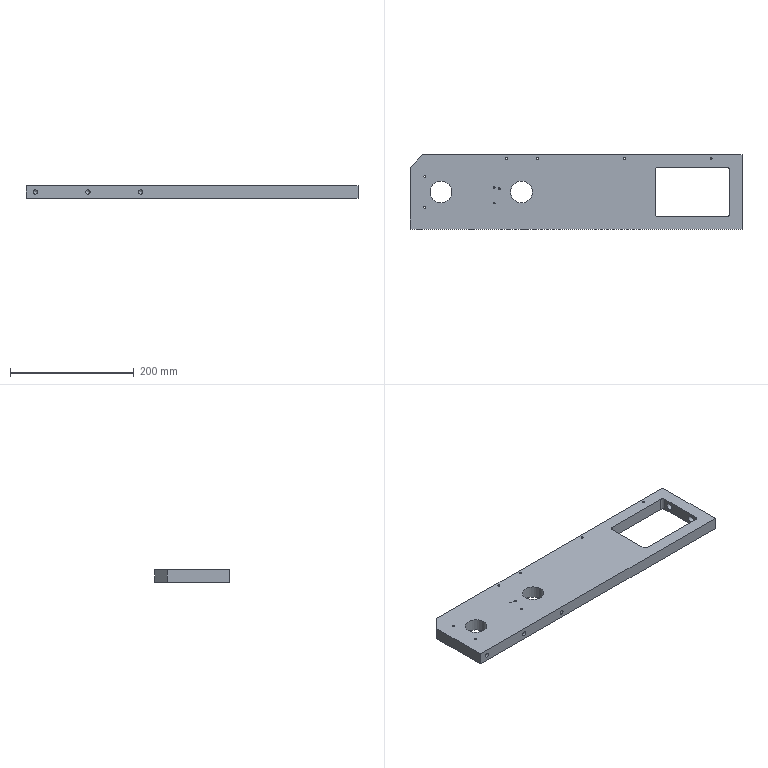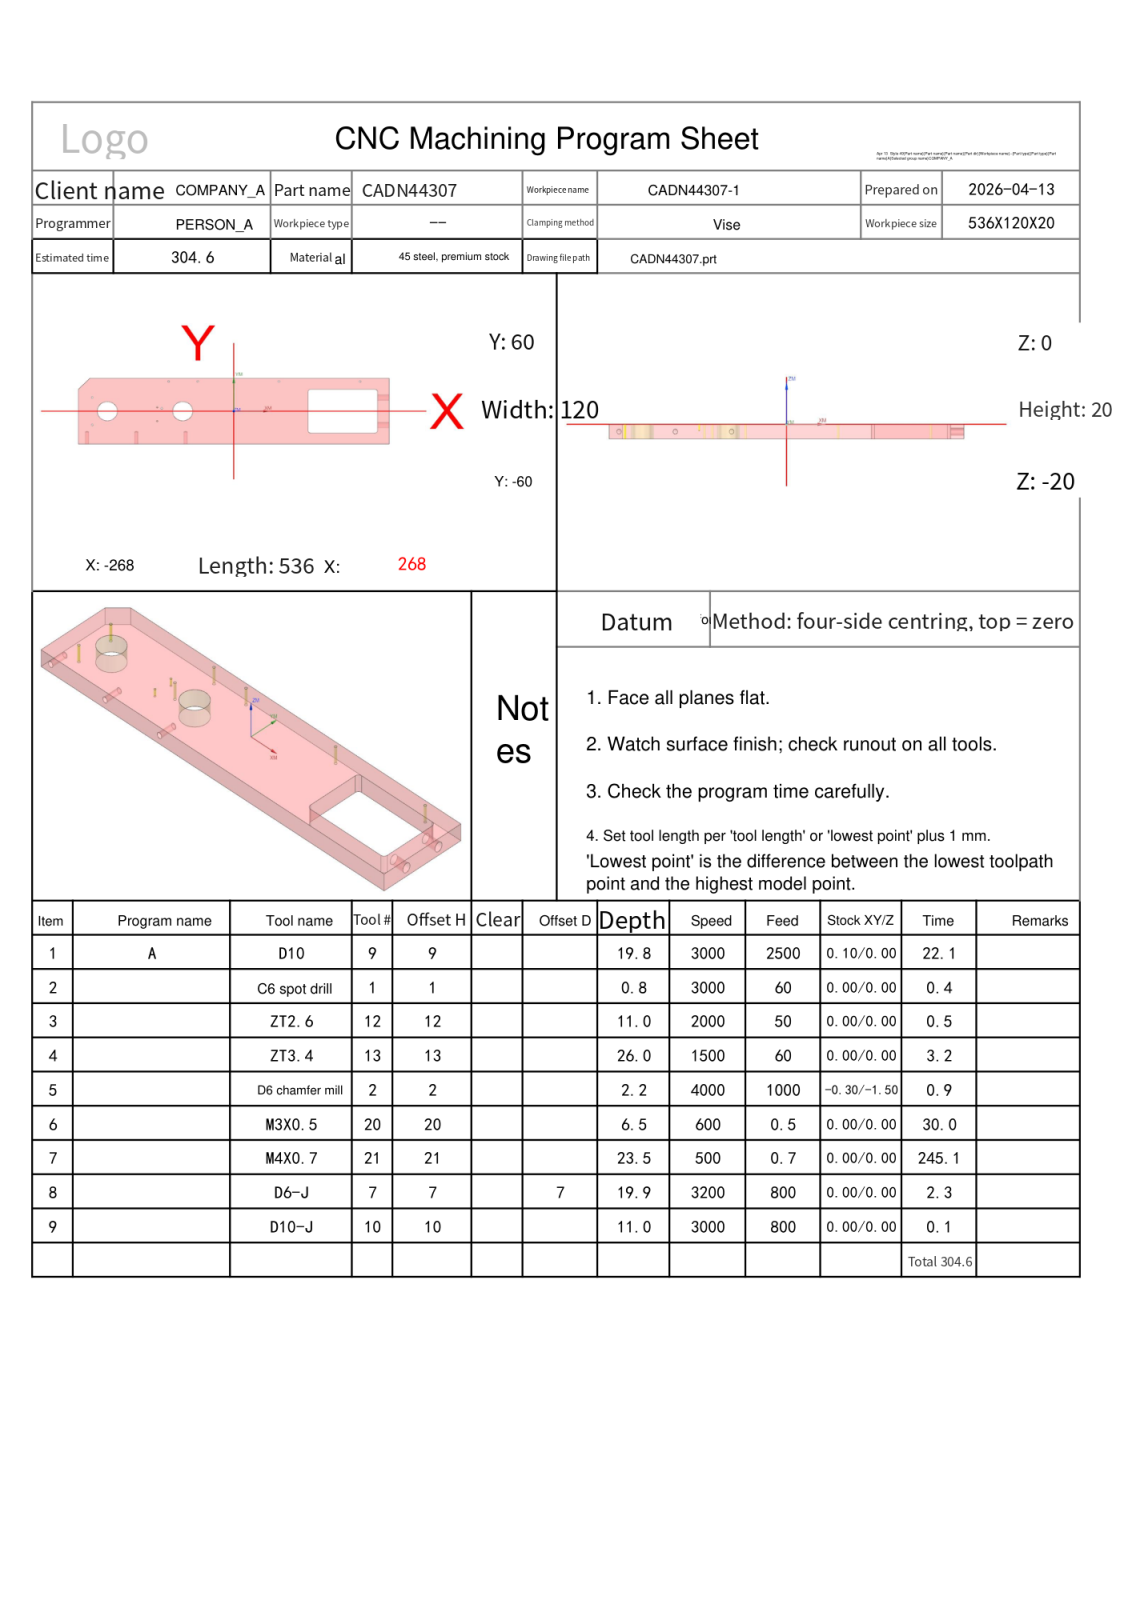NC program | NX | posted by the shop | part box 536 x 120 x 20 mm
Whole program, first 1074 of 1856 lines:
%
O0001
(Machine time: 567.38 MIN)
(===Total Tool:9===)
(T9=D10     D=10.  R=0.   D-  H09 Z=-19.8 )
(T1=C6 spot drill   D=6.   R=0.   D-  H01 Z=-0.8  )
(T12=ZT2.6  D=2.6  DR_a=118 D-  H12 Z=-11.  )
(T13=ZT3.4  D=3.4  DR_a=118 D-  H13 Z=-26.  )
(T2=D6 chamfer mill   D=6.   R=0.   D-  H02 Z=-2.2  )
(T20=M3X0.5 D=2.5  DR_a=180 D-  H20 Z=-6.5  )
(T21=M4X0.7 D=3.3  DR_a=180 D-  H21 Z=-23.5 )
(T7=D6-J    D=6.   R=0.   D7  H07 Z=-19.85)
(T10=D10-J  D=10.  R=0.   D-  H10 Z=-11.  )
G80 G90 G17 G49 G40
G91 G28 Z0
M01
N1 T09 M06
(D10  D=10. R=0. H=09 ce=0.10 di=0.00)
G00 G90 G54 X-230.4 Y0.0 M03 S3000
G43 H09 Z20.
M08
Z.5
G03 X-218. Y-12.4 Z.45 I12.4 J0.0 F2500.
X-205.6 Y0.0 Z.4 I0.0 J12.4
X-218. Y12.4 Z.351 I-12.4 J0.0
X-230.4 Y0.0 Z.301 I0.0 J-12.4
X-218. Y-12.4 Z.251 I12.4 J0.0
X-205.6 Y0.0 Z.201 I0.0 J12.4
X-218. Y12.4 Z.152 I-12.4 J0.0
X-230.4 Y0.0 Z.102 I0.0 J-12.4
X-218. Y-12.4 Z.052 I12.4 J0.0
X-205.6 Y0.0 Z.002 I0.0 J12.4
X-218. Y12.4 Z-.047 I-12.4 J0.0
X-230.4 Y0.0 Z-.097 I0.0 J-12.4
X-218. Y-12.4 Z-.147 I12.4 J0.0
X-205.6 Y0.0 Z-.197 I0.0 J12.4
X-218. Y12.4 Z-.246 I-12.4 J0.0
X-230.4 Y0.0 Z-.296 I0.0 J-12.4
X-218. Y-12.4 Z-.346 I12.4 J0.0
X-205.6 Y0.0 Z-.396 I0.0 J12.4
X-218. Y12.4 Z-.445 I-12.4 J0.0
X-230.4 Y0.0 Z-.495 I0.0 J-12.4
X-218. Y-12.4 Z-.545 I12.4 J0.0
X-205.6 Y0.0 Z-.595 I0.0 J12.4
X-218. Y12.4 Z-.644 I-12.4 J0.0
X-230.4 Y0.0 Z-.694 I0.0 J-12.4
X-218. Y-12.4 Z-.744 I12.4 J0.0
X-205.6 Y0.0 Z-.794 I0.0 J12.4
X-218. Y12.4 Z-.843 I-12.4 J0.0
X-230.4 Y0.0 Z-.893 I0.0 J-12.4
X-218. Y-12.4 Z-.943 I12.4 J0.0
X-205.6 Y0.0 Z-.993 I0.0 J12.4
X-218. Y12.4 Z-1.042 I-12.4 J0.0
X-230.4 Y0.0 Z-1.092 I0.0 J-12.4
X-218. Y-12.4 Z-1.142 I12.4 J0.0
X-205.6 Y0.0 Z-1.192 I0.0 J12.4
X-218. Y12.4 Z-1.241 I-12.4 J0.0
X-230.4 Y0.0 Z-1.291 I0.0 J-12.4
X-218. Y-12.4 Z-1.341 I12.4 J0.0
X-205.6 Y0.0 Z-1.391 I0.0 J12.4
X-218. Y12.4 Z-1.44 I-12.4 J0.0
X-230.4 Y0.0 Z-1.49 I0.0 J-12.4
X-218. Y-12.4 Z-1.54 I12.4 J0.0
X-205.6 Y0.0 Z-1.59 I0.0 J12.4
X-218. Y12.4 Z-1.639 I-12.4 J0.0
X-230.4 Y0.0 Z-1.689 I0.0 J-12.4
X-218. Y-12.4 Z-1.739 I12.4 J0.0
X-205.6 Y0.0 Z-1.789 I0.0 J12.4
X-218. Y12.4 Z-1.838 I-12.4 J0.0
X-230.4 Y0.0 Z-1.888 I0.0 J-12.4
X-218. Y-12.4 Z-1.938 I12.4 J0.0
X-205.6 Y0.0 Z-1.988 I0.0 J12.4
X-218. Y12.4 Z-2.038 I-12.4 J0.0
X-230.4 Y0.0 Z-2.087 I0.0 J-12.4
X-218. Y-12.4 Z-2.137 I12.4 J0.0
X-205.6 Y0.0 Z-2.187 I0.0 J12.4
X-218. Y12.4 Z-2.237 I-12.4 J0.0
X-230.4 Y0.0 Z-2.286 I0.0 J-12.4
X-218. Y-12.4 Z-2.336 I12.4 J0.0
X-205.6 Y0.0 Z-2.386 I0.0 J12.4
X-218. Y12.4 Z-2.436 I-12.4 J0.0
X-230.4 Y0.0 Z-2.485 I0.0 J-12.4
X-218. Y-12.4 Z-2.535 I12.4 J0.0
X-205.6 Y0.0 Z-2.585 I0.0 J12.4
X-218. Y12.4 Z-2.635 I-12.4 J0.0
X-230.4 Y0.0 Z-2.684 I0.0 J-12.4
X-218. Y-12.4 Z-2.734 I12.4 J0.0
X-205.6 Y0.0 Z-2.784 I0.0 J12.4
X-218. Y12.4 Z-2.834 I-12.4 J0.0
X-230.4 Y0.0 Z-2.883 I0.0 J-12.4
X-218. Y-12.4 Z-2.933 I12.4 J0.0
X-205.6 Y0.0 Z-2.983 I0.0 J12.4
X-218. Y12.4 Z-3.033 I-12.4 J0.0
X-230.4 Y0.0 Z-3.082 I0.0 J-12.4
X-218. Y-12.4 Z-3.132 I12.4 J0.0
X-205.6 Y0.0 Z-3.182 I0.0 J12.4
X-218. Y12.4 Z-3.232 I-12.4 J0.0
X-230.4 Y0.0 Z-3.281 I0.0 J-12.4
X-218. Y-12.4 Z-3.331 I12.4 J0.0
X-205.6 Y0.0 Z-3.381 I0.0 J12.4
X-218. Y12.4 Z-3.431 I-12.4 J0.0
X-230.4 Y0.0 Z-3.48 I0.0 J-12.4
X-218. Y-12.4 Z-3.53 I12.4 J0.0
X-205.6 Y0.0 Z-3.58 I0.0 J12.4
X-218. Y12.4 Z-3.63 I-12.4 J0.0
X-230.4 Y0.0 Z-3.679 I0.0 J-12.4
X-218. Y-12.4 Z-3.729 I12.4 J0.0
X-205.6 Y0.0 Z-3.779 I0.0 J12.4
X-218. Y12.4 Z-3.829 I-12.4 J0.0
X-230.4 Y0.0 Z-3.878 I0.0 J-12.4
X-218. Y-12.4 Z-3.928 I12.4 J0.0
X-205.6 Y0.0 Z-3.978 I0.0 J12.4
X-218. Y12.4 Z-4.028 I-12.4 J0.0
X-230.4 Y0.0 Z-4.077 I0.0 J-12.4
X-218. Y-12.4 Z-4.127 I12.4 J0.0
X-205.6 Y0.0 Z-4.177 I0.0 J12.4
X-218. Y12.4 Z-4.227 I-12.4 J0.0
X-230.4 Y0.0 Z-4.276 I0.0 J-12.4
X-218. Y-12.4 Z-4.326 I12.4 J0.0
X-205.6 Y0.0 Z-4.376 I0.0 J12.4
X-218. Y12.4 Z-4.426 I-12.4 J0.0
X-230.4 Y0.0 Z-4.475 I0.0 J-12.4
X-218. Y-12.4 Z-4.525 I12.4 J0.0
X-205.6 Y0.0 Z-4.575 I0.0 J12.4
X-218. Y12.4 Z-4.625 I-12.4 J0.0
X-230.4 Y0.0 Z-4.675 I0.0 J-12.4
X-218. Y-12.4 Z-4.724 I12.4 J0.0
X-205.6 Y0.0 Z-4.774 I0.0 J12.4
X-218. Y12.4 Z-4.824 I-12.4 J0.0
X-230.4 Y0.0 Z-4.874 I0.0 J-12.4
X-218. Y-12.4 Z-4.923 I12.4 J0.0
X-205.6 Y0.0 Z-4.973 I0.0 J12.4
X-218. Y12.4 Z-5.023 I-12.4 J0.0
X-230.4 Y0.0 Z-5.073 I0.0 J-12.4
X-218. Y-12.4 Z-5.122 I12.4 J0.0
X-205.6 Y0.0 Z-5.172 I0.0 J12.4
X-218. Y12.4 Z-5.222 I-12.4 J0.0
X-230.4 Y0.0 Z-5.272 I0.0 J-12.4
X-218. Y-12.4 Z-5.321 I12.4 J0.0
X-205.6 Y0.0 Z-5.371 I0.0 J12.4
X-218. Y12.4 Z-5.421 I-12.4 J0.0
X-230.4 Y0.0 Z-5.471 I0.0 J-12.4
X-218. Y-12.4 Z-5.52 I12.4 J0.0
X-205.6 Y0.0 Z-5.57 I0.0 J12.4
X-218. Y12.4 Z-5.62 I-12.4 J0.0
X-230.4 Y0.0 Z-5.67 I0.0 J-12.4
X-218. Y-12.4 Z-5.719 I12.4 J0.0
X-205.6 Y0.0 Z-5.769 I0.0 J12.4
X-218. Y12.4 Z-5.819 I-12.4 J0.0
X-230.4 Y0.0 Z-5.869 I0.0 J-12.4
X-218. Y-12.4 Z-5.918 I12.4 J0.0
X-205.6 Y0.0 Z-5.968 I0.0 J12.4
X-218. Y12.4 Z-6.018 I-12.4 J0.0
X-230.4 Y0.0 Z-6.068 I0.0 J-12.4
X-218. Y-12.4 Z-6.117 I12.4 J0.0
X-205.6 Y0.0 Z-6.167 I0.0 J12.4
X-218. Y12.4 Z-6.217 I-12.4 J0.0
X-230.4 Y0.0 Z-6.267 I0.0 J-12.4
X-218. Y-12.4 Z-6.316 I12.4 J0.0
X-205.6 Y0.0 Z-6.366 I0.0 J12.4
X-218. Y12.4 Z-6.416 I-12.4 J0.0
X-230.4 Y0.0 Z-6.466 I0.0 J-12.4
X-218. Y-12.4 Z-6.515 I12.4 J0.0
X-205.6 Y0.0 Z-6.565 I0.0 J12.4
X-218. Y12.4 Z-6.615 I-12.4 J0.0
X-230.4 Y0.0 Z-6.665 I0.0 J-12.4
X-218. Y-12.4 Z-6.714 I12.4 J0.0
X-205.6 Y0.0 Z-6.764 I0.0 J12.4
X-218. Y12.4 Z-6.814 I-12.4 J0.0
X-230.4 Y0.0 Z-6.864 I0.0 J-12.4
X-218. Y-12.4 Z-6.913 I12.4 J0.0
X-205.6 Y0.0 Z-6.963 I0.0 J12.4
X-218. Y12.4 Z-7.013 I-12.4 J0.0
X-230.4 Y0.0 Z-7.063 I0.0 J-12.4
X-218. Y-12.4 Z-7.113 I12.4 J0.0
X-205.6 Y0.0 Z-7.162 I0.0 J12.4
X-218. Y12.4 Z-7.212 I-12.4 J0.0
X-230.4 Y0.0 Z-7.262 I0.0 J-12.4
X-218. Y-12.4 Z-7.312 I12.4 J0.0
X-205.6 Y0.0 Z-7.361 I0.0 J12.4
X-218. Y12.4 Z-7.411 I-12.4 J0.0
X-230.4 Y0.0 Z-7.461 I0.0 J-12.4
X-218. Y-12.4 Z-7.511 I12.4 J0.0
X-205.6 Y0.0 Z-7.56 I0.0 J12.4
X-218. Y12.4 Z-7.61 I-12.4 J0.0
X-230.4 Y0.0 Z-7.66 I0.0 J-12.4
X-218. Y-12.4 Z-7.71 I12.4 J0.0
X-205.6 Y0.0 Z-7.759 I0.0 J12.4
X-218. Y12.4 Z-7.809 I-12.4 J0.0
X-230.4 Y0.0 Z-7.859 I0.0 J-12.4
X-218. Y-12.4 Z-7.909 I12.4 J0.0
X-205.6 Y0.0 Z-7.958 I0.0 J12.4
X-218. Y12.4 Z-8.008 I-12.4 J0.0
X-230.4 Y0.0 Z-8.058 I0.0 J-12.4
X-218. Y-12.4 Z-8.108 I12.4 J0.0
X-205.6 Y0.0 Z-8.157 I0.0 J12.4
X-218. Y12.4 Z-8.207 I-12.4 J0.0
X-230.4 Y0.0 Z-8.257 I0.0 J-12.4
X-218. Y-12.4 Z-8.307 I12.4 J0.0
X-205.6 Y0.0 Z-8.356 I0.0 J12.4
X-218. Y12.4 Z-8.406 I-12.4 J0.0
X-230.4 Y0.0 Z-8.456 I0.0 J-12.4
X-218. Y-12.4 Z-8.506 I12.4 J0.0
X-205.6 Y0.0 Z-8.555 I0.0 J12.4
X-218. Y12.4 Z-8.605 I-12.4 J0.0
X-230.4 Y0.0 Z-8.655 I0.0 J-12.4
X-218. Y-12.4 Z-8.705 I12.4 J0.0
X-205.6 Y0.0 Z-8.754 I0.0 J12.4
X-218. Y12.4 Z-8.804 I-12.4 J0.0
X-230.4 Y0.0 Z-8.854 I0.0 J-12.4
X-218. Y-12.4 Z-8.904 I12.4 J0.0
X-205.6 Y0.0 Z-8.953 I0.0 J12.4
X-218. Y12.4 Z-9.003 I-12.4 J0.0
X-230.4 Y0.0 Z-9.053 I0.0 J-12.4
X-218. Y-12.4 Z-9.103 I12.4 J0.0
X-205.6 Y0.0 Z-9.152 I0.0 J12.4
X-218. Y12.4 Z-9.202 I-12.4 J0.0
X-230.4 Y0.0 Z-9.252 I0.0 J-12.4
X-218. Y-12.4 Z-9.302 I12.4 J0.0
X-205.6 Y0.0 Z-9.351 I0.0 J12.4
X-218. Y12.4 Z-9.401 I-12.4 J0.0
X-230.4 Y0.0 Z-9.451 I0.0 J-12.4
X-218. Y-12.4 Z-9.501 I12.4 J0.0
X-205.6 Y0.0 Z-9.55 I0.0 J12.4
X-218. Y12.4 Z-9.6 I-12.4 J0.0
X-230.4 Y0.0 Z-9.65 I0.0 J-12.4
X-218. Y-12.4 Z-9.7 I12.4 J0.0
X-205.6 Y0.0 Z-9.75 I0.0 J12.4
X-218. Y12.4 Z-9.799 I-12.4 J0.0
X-230.4 Y0.0 Z-9.849 I0.0 J-12.4
X-218. Y-12.4 Z-9.899 I12.4 J0.0
X-205.6 Y0.0 Z-9.949 I0.0 J12.4
X-218. Y12.4 Z-9.998 I-12.4 J0.0
X-230.4 Y0.0 Z-10.048 I0.0 J-12.4
X-218. Y-12.4 Z-10.098 I12.4 J0.0
X-205.6 Y0.0 Z-10.148 I0.0 J12.4
X-218. Y12.4 Z-10.197 I-12.4 J0.0
X-230.4 Y0.0 Z-10.247 I0.0 J-12.4
X-218. Y-12.4 Z-10.297 I12.4 J0.0
X-205.6 Y0.0 Z-10.347 I0.0 J12.4
X-218. Y12.4 Z-10.396 I-12.4 J0.0
X-230.4 Y0.0 Z-10.446 I0.0 J-12.4
X-218. Y-12.4 Z-10.496 I12.4 J0.0
X-205.6 Y0.0 Z-10.546 I0.0 J12.4
X-218. Y12.4 Z-10.595 I-12.4 J0.0
X-230.4 Y0.0 Z-10.645 I0.0 J-12.4
X-218. Y-12.4 Z-10.695 I12.4 J0.0
X-205.6 Y0.0 Z-10.745 I0.0 J12.4
X-218. Y12.4 Z-10.794 I-12.4 J0.0
X-230.4 Y0.0 Z-10.844 I0.0 J-12.4
X-218. Y-12.4 Z-10.894 I12.4 J0.0
X-205.6 Y0.0 Z-10.944 I0.0 J12.4
X-218. Y12.4 Z-10.993 I-12.4 J0.0
X-230.4 Y0.0 Z-11.043 I0.0 J-12.4
X-218. Y-12.4 Z-11.093 I12.4 J0.0
X-205.6 Y0.0 Z-11.143 I0.0 J12.4
X-218. Y12.4 Z-11.192 I-12.4 J0.0
X-230.4 Y0.0 Z-11.242 I0.0 J-12.4
X-218. Y-12.4 Z-11.292 I12.4 J0.0
X-205.6 Y0.0 Z-11.342 I0.0 J12.4
X-218. Y12.4 Z-11.391 I-12.4 J0.0
X-230.4 Y0.0 Z-11.441 I0.0 J-12.4
X-218. Y-12.4 Z-11.491 I12.4 J0.0
X-205.6 Y0.0 Z-11.541 I0.0 J12.4
X-218. Y12.4 Z-11.59 I-12.4 J0.0
X-230.4 Y0.0 Z-11.64 I0.0 J-12.4
X-218. Y-12.4 Z-11.69 I12.4 J0.0
X-205.6 Y0.0 Z-11.74 I0.0 J12.4
X-218. Y12.4 Z-11.789 I-12.4 J0.0
X-230.4 Y0.0 Z-11.839 I0.0 J-12.4
X-218. Y-12.4 Z-11.889 I12.4 J0.0
X-205.6 Y0.0 Z-11.939 I0.0 J12.4
X-218. Y12.4 Z-11.988 I-12.4 J0.0
X-230.4 Y0.0 Z-12.038 I0.0 J-12.4
X-218. Y-12.4 Z-12.088 I12.4 J0.0
X-205.6 Y0.0 Z-12.138 I0.0 J12.4
X-218. Y12.4 Z-12.188 I-12.4 J0.0
X-230.4 Y0.0 Z-12.237 I0.0 J-12.4
X-218. Y-12.4 Z-12.287 I12.4 J0.0
X-205.6 Y0.0 Z-12.337 I0.0 J12.4
X-218. Y12.4 Z-12.387 I-12.4 J0.0
X-230.4 Y0.0 Z-12.436 I0.0 J-12.4
X-218. Y-12.4 Z-12.486 I12.4 J0.0
X-205.6 Y0.0 Z-12.536 I0.0 J12.4
X-218. Y12.4 Z-12.586 I-12.4 J0.0
X-230.4 Y0.0 Z-12.635 I0.0 J-12.4
X-218. Y-12.4 Z-12.685 I12.4 J0.0
X-205.6 Y0.0 Z-12.735 I0.0 J12.4
X-218. Y12.4 Z-12.785 I-12.4 J0.0
X-230.4 Y0.0 Z-12.834 I0.0 J-12.4
X-218. Y-12.4 Z-12.884 I12.4 J0.0
X-205.6 Y0.0 Z-12.934 I0.0 J12.4
X-218. Y12.4 Z-12.984 I-12.4 J0.0
X-230.4 Y0.0 Z-13.033 I0.0 J-12.4
X-218. Y-12.4 Z-13.083 I12.4 J0.0
X-205.6 Y0.0 Z-13.133 I0.0 J12.4
X-218. Y12.4 Z-13.183 I-12.4 J0.0
X-230.4 Y0.0 Z-13.232 I0.0 J-12.4
X-218. Y-12.4 Z-13.282 I12.4 J0.0
X-205.6 Y0.0 Z-13.332 I0.0 J12.4
X-218. Y12.4 Z-13.382 I-12.4 J0.0
X-230.4 Y0.0 Z-13.431 I0.0 J-12.4
X-218. Y-12.4 Z-13.481 I12.4 J0.0
X-205.6 Y0.0 Z-13.531 I0.0 J12.4
X-218. Y12.4 Z-13.581 I-12.4 J0.0
X-230.4 Y0.0 Z-13.63 I0.0 J-12.4
X-218. Y-12.4 Z-13.68 I12.4 J0.0
X-205.6 Y0.0 Z-13.73 I0.0 J12.4
X-218. Y12.4 Z-13.78 I-12.4 J0.0
X-230.4 Y0.0 Z-13.829 I0.0 J-12.4
X-218. Y-12.4 Z-13.879 I12.4 J0.0
X-205.6 Y0.0 Z-13.929 I0.0 J12.4
X-218. Y12.4 Z-13.979 I-12.4 J0.0
X-230.4 Y0.0 Z-14.028 I0.0 J-12.4
X-218. Y-12.4 Z-14.078 I12.4 J0.0
X-205.6 Y0.0 Z-14.128 I0.0 J12.4
X-218. Y12.4 Z-14.178 I-12.4 J0.0
X-230.4 Y0.0 Z-14.227 I0.0 J-12.4
X-218. Y-12.4 Z-14.277 I12.4 J0.0
X-205.6 Y0.0 Z-14.327 I0.0 J12.4
X-218. Y12.4 Z-14.377 I-12.4 J0.0
X-230.4 Y0.0 Z-14.426 I0.0 J-12.4
X-218. Y-12.4 Z-14.476 I12.4 J0.0
X-205.6 Y0.0 Z-14.526 I0.0 J12.4
X-218. Y12.4 Z-14.576 I-12.4 J0.0
X-230.4 Y0.0 Z-14.625 I0.0 J-12.4
X-218. Y-12.4 Z-14.675 I12.4 J0.0
X-205.6 Y0.0 Z-14.725 I0.0 J12.4
X-218. Y12.4 Z-14.775 I-12.4 J0.0
X-230.4 Y0.0 Z-14.825 I0.0 J-12.4
X-218. Y-12.4 Z-14.874 I12.4 J0.0
X-205.6 Y0.0 Z-14.924 I0.0 J12.4
X-218. Y12.4 Z-14.974 I-12.4 J0.0
X-230.4 Y0.0 Z-15.024 I0.0 J-12.4
X-218. Y-12.4 Z-15.073 I12.4 J0.0
X-205.6 Y0.0 Z-15.123 I0.0 J12.4
X-218. Y12.4 Z-15.173 I-12.4 J0.0
X-230.4 Y0.0 Z-15.223 I0.0 J-12.4
X-218. Y-12.4 Z-15.272 I12.4 J0.0
X-205.6 Y0.0 Z-15.322 I0.0 J12.4
X-218. Y12.4 Z-15.372 I-12.4 J0.0
X-230.4 Y0.0 Z-15.422 I0.0 J-12.4
X-218. Y-12.4 Z-15.471 I12.4 J0.0
X-205.6 Y0.0 Z-15.521 I0.0 J12.4
X-218. Y12.4 Z-15.571 I-12.4 J0.0
X-230.4 Y0.0 Z-15.621 I0.0 J-12.4
X-218. Y-12.4 Z-15.67 I12.4 J0.0
X-205.6 Y0.0 Z-15.72 I0.0 J12.4
X-218. Y12.4 Z-15.77 I-12.4 J0.0
X-230.4 Y0.0 Z-15.82 I0.0 J-12.4
X-218. Y-12.4 Z-15.869 I12.4 J0.0
X-205.6 Y0.0 Z-15.919 I0.0 J12.4
X-218. Y12.4 Z-15.969 I-12.4 J0.0
X-230.4 Y0.0 Z-16.019 I0.0 J-12.4
X-218. Y-12.4 Z-16.068 I12.4 J0.0
X-205.6 Y0.0 Z-16.118 I0.0 J12.4
X-218. Y12.4 Z-16.168 I-12.4 J0.0
X-230.4 Y0.0 Z-16.218 I0.0 J-12.4
X-218. Y-12.4 Z-16.267 I12.4 J0.0
X-205.6 Y0.0 Z-16.317 I0.0 J12.4
X-218. Y12.4 Z-16.367 I-12.4 J0.0
X-230.4 Y0.0 Z-16.417 I0.0 J-12.4
X-218. Y-12.4 Z-16.466 I12.4 J0.0
X-205.6 Y0.0 Z-16.516 I0.0 J12.4
X-218. Y12.4 Z-16.566 I-12.4 J0.0
X-230.4 Y0.0 Z-16.616 I0.0 J-12.4
X-218. Y-12.4 Z-16.665 I12.4 J0.0
X-205.6 Y0.0 Z-16.715 I0.0 J12.4
X-218. Y12.4 Z-16.765 I-12.4 J0.0
X-230.4 Y0.0 Z-16.815 I0.0 J-12.4
X-218. Y-12.4 Z-16.864 I12.4 J0.0
X-205.6 Y0.0 Z-16.914 I0.0 J12.4
X-218. Y12.4 Z-16.964 I-12.4 J0.0
X-230.4 Y0.0 Z-17.014 I0.0 J-12.4
X-218. Y-12.4 Z-17.063 I12.4 J0.0
X-205.6 Y0.0 Z-17.113 I0.0 J12.4
X-218. Y12.4 Z-17.163 I-12.4 J0.0
X-230.4 Y0.0 Z-17.213 I0.0 J-12.4
X-218. Y-12.4 Z-17.263 I12.4 J0.0
X-205.6 Y0.0 Z-17.312 I0.0 J12.4
X-218. Y12.4 Z-17.362 I-12.4 J0.0
X-230.4 Y0.0 Z-17.412 I0.0 J-12.4
X-218. Y-12.4 Z-17.462 I12.4 J0.0
X-205.6 Y0.0 Z-17.511 I0.0 J12.4
X-218. Y12.4 Z-17.561 I-12.4 J0.0
X-230.4 Y0.0 Z-17.611 I0.0 J-12.4
X-218. Y-12.4 Z-17.661 I12.4 J0.0
X-205.6 Y0.0 Z-17.71 I0.0 J12.4
X-218. Y12.4 Z-17.76 I-12.4 J0.0
X-230.4 Y0.0 Z-17.81 I0.0 J-12.4
X-218. Y-12.4 Z-17.86 I12.4 J0.0
X-205.6 Y0.0 Z-17.909 I0.0 J12.4
X-218. Y12.4 Z-17.959 I-12.4 J0.0
X-230.4 Y0.0 Z-18.009 I0.0 J-12.4
X-218. Y-12.4 Z-18.059 I12.4 J0.0
X-205.6 Y0.0 Z-18.108 I0.0 J12.4
X-218. Y12.4 Z-18.158 I-12.4 J0.0
X-230.4 Y0.0 Z-18.208 I0.0 J-12.4
X-218. Y-12.4 Z-18.258 I12.4 J0.0
X-205.6 Y0.0 Z-18.307 I0.0 J12.4
X-218. Y12.4 Z-18.357 I-12.4 J0.0
X-230.4 Y0.0 Z-18.407 I0.0 J-12.4
X-218. Y-12.4 Z-18.457 I12.4 J0.0
X-205.6 Y0.0 Z-18.506 I0.0 J12.4
X-218. Y12.4 Z-18.556 I-12.4 J0.0
X-230.4 Y0.0 Z-18.606 I0.0 J-12.4
X-218. Y-12.4 Z-18.656 I12.4 J0.0
X-205.6 Y0.0 Z-18.705 I0.0 J12.4
X-218. Y12.4 Z-18.755 I-12.4 J0.0
X-230.4 Y0.0 Z-18.805 I0.0 J-12.4
X-218. Y-12.4 Z-18.855 I12.4 J0.0
X-205.6 Y0.0 Z-18.904 I0.0 J12.4
X-218. Y12.4 Z-18.954 I-12.4 J0.0
X-230.4 Y0.0 Z-19.004 I0.0 J-12.4
X-218. Y-12.4 Z-19.054 I12.4 J0.0
X-205.6 Y0.0 Z-19.103 I0.0 J12.4
X-218. Y12.4 Z-19.153 I-12.4 J0.0
X-230.4 Y0.0 Z-19.203 I0.0 J-12.4
X-218. Y-12.4 Z-19.253 I12.4 J0.0
X-205.6 Y0.0 Z-19.302 I0.0 J12.4
X-218. Y12.4 Z-19.352 I-12.4 J0.0
X-230.4 Y0.0 Z-19.402 I0.0 J-12.4
X-218. Y-12.4 Z-19.452 I12.4 J0.0
X-205.6 Y0.0 Z-19.501 I0.0 J12.4
X-218. Y12.4 Z-19.551 I-12.4 J0.0
X-230.4 Y0.0 Z-19.601 I0.0 J-12.4
X-218. Y-12.4 Z-19.651 I12.4 J0.0
X-205.6 Y0.0 Z-19.7 I0.0 J12.4
X-218. Y12.4 Z-19.75 I-12.4 J0.0
X-230.4 Y0.0 Z-19.8 I0.0 J-12.4
X-218. Y-12.4 I12.4 J0.0
X-205.6 Y0.0 I0.0 J12.4
X-218. Y12.4 I-12.4 J0.0
X-230.4 Y0.0 I0.0 J-12.4
X-230.39 Y-.5 I12.4 J0.0
G01 Z-18.8
G00 Z20.
X-88. Y-12.4
Z.5
G03 X-75.6 Y0.0 Z.45 I0.0 J12.4
X-88. Y12.4 Z.4 I-12.4 J0.0
X-100.4 Y0.0 Z.351 I0.0 J-12.4
X-95.145 Y-10.135 Z.32 I12.4 J0.0
X-88. Y-12.4 Z.301 I7.145 J10.135
X-75.6 Y0.0 Z.251 I0.0 J12.4
X-88. Y12.4 Z.201 I-12.4 J0.0
X-100.4 Y0.0 Z.152 I0.0 J-12.4
X-95.145 Y-10.135 Z.121 I12.4 J0.0
X-88. Y-12.4 Z.102 I7.145 J10.135
X-75.6 Y0.0 Z.052 I0.0 J12.4
X-88. Y12.4 Z.002 I-12.4 J0.0
X-100.4 Y0.0 Z-.047 I0.0 J-12.4
X-95.145 Y-10.135 Z-.078 I12.4 J0.0
X-88. Y-12.4 Z-.097 I7.145 J10.135
X-75.6 Y0.0 Z-.147 I0.0 J12.4
X-88. Y12.4 Z-.197 I-12.4 J0.0
X-100.4 Y0.0 Z-.246 I0.0 J-12.4
X-95.145 Y-10.135 Z-.277 I12.4 J0.0
X-88. Y-12.4 Z-.296 I7.145 J10.135
X-75.6 Y0.0 Z-.346 I0.0 J12.4
X-88. Y12.4 Z-.396 I-12.4 J0.0
X-100.4 Y0.0 Z-.445 I0.0 J-12.4
X-95.145 Y-10.135 Z-.476 I12.4 J0.0
X-88. Y-12.4 Z-.495 I7.145 J10.135
X-75.6 Y0.0 Z-.545 I0.0 J12.4
X-88. Y12.4 Z-.595 I-12.4 J0.0
X-100.4 Y0.0 Z-.644 I0.0 J-12.4
X-95.145 Y-10.135 Z-.675 I12.4 J0.0
X-88. Y-12.4 Z-.694 I7.145 J10.135
X-75.6 Y0.0 Z-.744 I0.0 J12.4
X-88. Y12.4 Z-.794 I-12.4 J0.0
X-100.4 Y0.0 Z-.843 I0.0 J-12.4
X-95.145 Y-10.135 Z-.874 I12.4 J0.0
X-88. Y-12.4 Z-.893 I7.145 J10.135
X-75.6 Y0.0 Z-.943 I0.0 J12.4
X-88. Y12.4 Z-.993 I-12.4 J0.0
X-100.4 Y0.0 Z-1.042 I0.0 J-12.4
X-95.145 Y-10.135 Z-1.073 I12.4 J0.0
X-88. Y-12.4 Z-1.092 I7.145 J10.135
X-75.6 Y0.0 Z-1.142 I0.0 J12.4
X-88. Y12.4 Z-1.192 I-12.4 J0.0
X-100.4 Y0.0 Z-1.241 I0.0 J-12.4
X-95.145 Y-10.135 Z-1.272 I12.4 J0.0
X-88. Y-12.4 Z-1.291 I7.145 J10.135
X-75.6 Y0.0 Z-1.341 I0.0 J12.4
X-88. Y12.4 Z-1.391 I-12.4 J0.0
X-100.4 Y0.0 Z-1.44 I0.0 J-12.4
X-95.145 Y-10.135 Z-1.471 I12.4 J0.0
X-88. Y-12.4 Z-1.49 I7.145 J10.135
X-75.6 Y0.0 Z-1.54 I0.0 J12.4
X-88. Y12.4 Z-1.59 I-12.4 J0.0
X-100.4 Y0.0 Z-1.639 I0.0 J-12.4
X-95.145 Y-10.135 Z-1.67 I12.4 J0.0
X-88. Y-12.4 Z-1.689 I7.145 J10.135
X-75.6 Y0.0 Z-1.739 I0.0 J12.4
X-88. Y12.4 Z-1.789 I-12.4 J0.0
X-100.4 Y0.0 Z-1.838 I0.0 J-12.4
X-95.145 Y-10.135 Z-1.869 I12.4 J0.0
X-88. Y-12.4 Z-1.888 I7.145 J10.135
X-75.6 Y0.0 Z-1.938 I0.0 J12.4
X-88. Y12.4 Z-1.988 I-12.4 J0.0
X-100.4 Y0.0 Z-2.038 I0.0 J-12.4
X-95.145 Y-10.135 Z-2.068 I12.4 J0.0
X-88. Y-12.4 Z-2.087 I7.145 J10.135
X-75.6 Y0.0 Z-2.137 I0.0 J12.4
X-88. Y12.4 Z-2.187 I-12.4 J0.0
X-100.4 Y0.0 Z-2.237 I0.0 J-12.4
X-95.145 Y-10.135 Z-2.267 I12.4 J0.0
X-88. Y-12.4 Z-2.286 I7.145 J10.135
X-75.6 Y0.0 Z-2.336 I0.0 J12.4
X-88. Y12.4 Z-2.386 I-12.4 J0.0
X-100.4 Y0.0 Z-2.436 I0.0 J-12.4
X-95.145 Y-10.135 Z-2.466 I12.4 J0.0
X-88. Y-12.4 Z-2.485 I7.145 J10.135
X-75.6 Y0.0 Z-2.535 I0.0 J12.4
X-88. Y12.4 Z-2.585 I-12.4 J0.0
X-100.4 Y0.0 Z-2.635 I0.0 J-12.4
X-95.145 Y-10.135 Z-2.665 I12.4 J0.0
X-88. Y-12.4 Z-2.684 I7.145 J10.135
X-75.6 Y0.0 Z-2.734 I0.0 J12.4
X-88. Y12.4 Z-2.784 I-12.4 J0.0
X-100.4 Y0.0 Z-2.834 I0.0 J-12.4
X-95.145 Y-10.135 Z-2.864 I12.4 J0.0
X-88. Y-12.4 Z-2.883 I7.145 J10.135
X-75.6 Y0.0 Z-2.933 I0.0 J12.4
X-88. Y12.4 Z-2.983 I-12.4 J0.0
X-100.4 Y0.0 Z-3.033 I0.0 J-12.4
X-95.145 Y-10.135 Z-3.063 I12.4 J0.0
X-88. Y-12.4 Z-3.082 I7.145 J10.135
X-75.6 Y0.0 Z-3.132 I0.0 J12.4
X-88. Y12.4 Z-3.182 I-12.4 J0.0
X-100.4 Y0.0 Z-3.232 I0.0 J-12.4
X-95.145 Y-10.135 Z-3.262 I12.4 J0.0
X-88. Y-12.4 Z-3.281 I7.145 J10.135
X-75.6 Y0.0 Z-3.331 I0.0 J12.4
X-88. Y12.4 Z-3.381 I-12.4 J0.0
X-100.4 Y0.0 Z-3.431 I0.0 J-12.4
X-95.145 Y-10.135 Z-3.461 I12.4 J0.0
X-88. Y-12.4 Z-3.48 I7.145 J10.135
X-75.6 Y0.0 Z-3.53 I0.0 J12.4
X-88. Y12.4 Z-3.58 I-12.4 J0.0
X-100.4 Y0.0 Z-3.63 I0.0 J-12.4
X-95.145 Y-10.135 Z-3.66 I12.4 J0.0
X-88. Y-12.4 Z-3.679 I7.145 J10.135
X-75.6 Y0.0 Z-3.729 I0.0 J12.4
X-88. Y12.4 Z-3.779 I-12.4 J0.0
X-100.4 Y0.0 Z-3.829 I0.0 J-12.4
X-95.145 Y-10.135 Z-3.859 I12.4 J0.0
X-88. Y-12.4 Z-3.878 I7.145 J10.135
X-75.6 Y0.0 Z-3.928 I0.0 J12.4
X-88. Y12.4 Z-3.978 I-12.4 J0.0
X-100.4 Y0.0 Z-4.028 I0.0 J-12.4
X-95.145 Y-10.135 Z-4.058 I12.4 J0.0
X-88. Y-12.4 Z-4.077 I7.145 J10.135
X-75.6 Y0.0 Z-4.127 I0.0 J12.4
X-88. Y12.4 Z-4.177 I-12.4 J0.0
X-100.4 Y0.0 Z-4.227 I0.0 J-12.4
X-95.145 Y-10.135 Z-4.257 I12.4 J0.0
X-88. Y-12.4 Z-4.276 I7.145 J10.135
X-75.6 Y0.0 Z-4.326 I0.0 J12.4
X-88. Y12.4 Z-4.376 I-12.4 J0.0
X-100.4 Y0.0 Z-4.426 I0.0 J-12.4
X-95.145 Y-10.135 Z-4.456 I12.4 J0.0
X-88. Y-12.4 Z-4.475 I7.145 J10.135
X-75.6 Y0.0 Z-4.525 I0.0 J12.4
X-88. Y12.4 Z-4.575 I-12.4 J0.0
X-100.4 Y0.0 Z-4.625 I0.0 J-12.4
X-95.145 Y-10.135 Z-4.655 I12.4 J0.0
X-88. Y-12.4 Z-4.675 I7.145 J10.135
X-75.6 Y0.0 Z-4.724 I0.0 J12.4
X-88. Y12.4 Z-4.774 I-12.4 J0.0
X-100.4 Y0.0 Z-4.824 I0.0 J-12.4
X-95.145 Y-10.135 Z-4.854 I12.4 J0.0
X-88. Y-12.4 Z-4.874 I7.145 J10.135
X-75.6 Y0.0 Z-4.923 I0.0 J12.4
X-88. Y12.4 Z-4.973 I-12.4 J0.0
X-100.4 Y0.0 Z-5.023 I0.0 J-12.4
X-95.145 Y-10.135 Z-5.053 I12.4 J0.0
X-88. Y-12.4 Z-5.073 I7.145 J10.135
X-75.6 Y0.0 Z-5.122 I0.0 J12.4
X-88. Y12.4 Z-5.172 I-12.4 J0.0
X-100.4 Y0.0 Z-5.222 I0.0 J-12.4
X-95.145 Y-10.135 Z-5.252 I12.4 J0.0
X-88. Y-12.4 Z-5.272 I7.145 J10.135
X-75.6 Y0.0 Z-5.321 I0.0 J12.4
X-88. Y12.4 Z-5.371 I-12.4 J0.0
X-100.4 Y0.0 Z-5.421 I0.0 J-12.4
X-95.145 Y-10.135 Z-5.451 I12.4 J0.0
X-88. Y-12.4 Z-5.471 I7.145 J10.135
X-75.6 Y0.0 Z-5.52 I0.0 J12.4
X-88. Y12.4 Z-5.57 I-12.4 J0.0
X-100.4 Y0.0 Z-5.62 I0.0 J-12.4
X-95.145 Y-10.135 Z-5.65 I12.4 J0.0
X-88. Y-12.4 Z-5.67 I7.145 J10.135
X-75.6 Y0.0 Z-5.719 I0.0 J12.4
X-88. Y12.4 Z-5.769 I-12.4 J0.0
X-100.4 Y0.0 Z-5.819 I0.0 J-12.4
X-95.145 Y-10.135 Z-5.849 I12.4 J0.0
X-88. Y-12.4 Z-5.869 I7.145 J10.135
X-75.6 Y0.0 Z-5.918 I0.0 J12.4
X-88. Y12.4 Z-5.968 I-12.4 J0.0
X-100.4 Y0.0 Z-6.018 I0.0 J-12.4
X-95.145 Y-10.135 Z-6.048 I12.4 J0.0
X-88. Y-12.4 Z-6.068 I7.145 J10.135
X-75.6 Y0.0 Z-6.117 I0.0 J12.4
X-88. Y12.4 Z-6.167 I-12.4 J0.0
X-100.4 Y0.0 Z-6.217 I0.0 J-12.4
X-95.145 Y-10.135 Z-6.247 I12.4 J0.0
X-88. Y-12.4 Z-6.267 I7.145 J10.135
X-75.6 Y0.0 Z-6.316 I0.0 J12.4
X-88. Y12.4 Z-6.366 I-12.4 J0.0
X-100.4 Y0.0 Z-6.416 I0.0 J-12.4
X-95.145 Y-10.135 Z-6.446 I12.4 J0.0
X-88. Y-12.4 Z-6.466 I7.145 J10.135
X-75.6 Y0.0 Z-6.515 I0.0 J12.4
X-88. Y12.4 Z-6.565 I-12.4 J0.0
X-100.4 Y0.0 Z-6.615 I0.0 J-12.4
X-95.145 Y-10.135 Z-6.645 I12.4 J0.0
X-88. Y-12.4 Z-6.665 I7.145 J10.135
X-75.6 Y0.0 Z-6.714 I0.0 J12.4
X-88. Y12.4 Z-6.764 I-12.4 J0.0
X-100.4 Y0.0 Z-6.814 I0.0 J-12.4
X-95.145 Y-10.135 Z-6.844 I12.4 J0.0
X-88. Y-12.4 Z-6.864 I7.145 J10.135
X-75.6 Y0.0 Z-6.913 I0.0 J12.4
X-88. Y12.4 Z-6.963 I-12.4 J0.0
X-100.4 Y0.0 Z-7.013 I0.0 J-12.4
X-95.145 Y-10.135 Z-7.043 I12.4 J0.0
X-88. Y-12.4 Z-7.063 I7.145 J10.135
X-75.6 Y0.0 Z-7.113 I0.0 J12.4
X-88. Y12.4 Z-7.162 I-12.4 J0.0
X-100.4 Y0.0 Z-7.212 I0.0 J-12.4
X-95.145 Y-10.135 Z-7.242 I12.4 J0.0
X-88. Y-12.4 Z-7.262 I7.145 J10.135
X-75.6 Y0.0 Z-7.312 I0.0 J12.4
X-88. Y12.4 Z-7.361 I-12.4 J0.0
X-100.4 Y0.0 Z-7.411 I0.0 J-12.4
X-95.145 Y-10.135 Z-7.441 I12.4 J0.0
X-88. Y-12.4 Z-7.461 I7.145 J10.135
X-75.6 Y0.0 Z-7.511 I0.0 J12.4
X-88. Y12.4 Z-7.56 I-12.4 J0.0
X-100.4 Y0.0 Z-7.61 I0.0 J-12.4
X-95.145 Y-10.135 Z-7.64 I12.4 J0.0
X-88. Y-12.4 Z-7.66 I7.145 J10.135
X-75.6 Y0.0 Z-7.71 I0.0 J12.4
X-88. Y12.4 Z-7.759 I-12.4 J0.0
X-100.4 Y0.0 Z-7.809 I0.0 J-12.4
X-95.145 Y-10.135 Z-7.839 I12.4 J0.0
X-88. Y-12.4 Z-7.859 I7.145 J10.135
X-75.6 Y0.0 Z-7.909 I0.0 J12.4
X-88. Y12.4 Z-7.958 I-12.4 J0.0
X-100.4 Y0.0 Z-8.008 I0.0 J-12.4
X-95.145 Y-10.135 Z-8.038 I12.4 J0.0
X-88. Y-12.4 Z-8.058 I7.145 J10.135
X-75.6 Y0.0 Z-8.108 I0.0 J12.4
X-88. Y12.4 Z-8.157 I-12.4 J0.0
X-100.4 Y0.0 Z-8.207 I0.0 J-12.4
X-95.145 Y-10.135 Z-8.237 I12.4 J0.0
X-88. Y-12.4 Z-8.257 I7.145 J10.135
X-75.6 Y0.0 Z-8.307 I0.0 J12.4
X-88. Y12.4 Z-8.356 I-12.4 J0.0
X-100.4 Y0.0 Z-8.406 I0.0 J-12.4
X-95.145 Y-10.135 Z-8.436 I12.4 J0.0
X-88. Y-12.4 Z-8.456 I7.145 J10.135
X-75.6 Y0.0 Z-8.506 I0.0 J12.4
X-88. Y12.4 Z-8.555 I-12.4 J0.0
X-100.4 Y0.0 Z-8.605 I0.0 J-12.4
X-95.145 Y-10.135 Z-8.635 I12.4 J0.0
X-88. Y-12.4 Z-8.655 I7.145 J10.135
X-75.6 Y0.0 Z-8.705 I0.0 J12.4
X-88. Y12.4 Z-8.754 I-12.4 J0.0
X-100.4 Y0.0 Z-8.804 I0.0 J-12.4
X-95.145 Y-10.135 Z-8.834 I12.4 J0.0
X-88. Y-12.4 Z-8.854 I7.145 J10.135
X-75.6 Y0.0 Z-8.904 I0.0 J12.4
X-88. Y12.4 Z-8.953 I-12.4 J0.0
X-100.4 Y0.0 Z-9.003 I0.0 J-12.4
X-95.145 Y-10.135 Z-9.033 I12.4 J0.0
X-88. Y-12.4 Z-9.053 I7.145 J10.135
X-75.6 Y0.0 Z-9.103 I0.0 J12.4
X-88. Y12.4 Z-9.152 I-12.4 J0.0
X-100.4 Y0.0 Z-9.202 I0.0 J-12.4
X-95.145 Y-10.135 Z-9.233 I12.4 J0.0
X-88. Y-12.4 Z-9.252 I7.145 J10.135
X-75.6 Y0.0 Z-9.302 I0.0 J12.4
X-88. Y12.4 Z-9.351 I-12.4 J0.0
X-100.4 Y0.0 Z-9.401 I0.0 J-12.4
X-95.145 Y-10.135 Z-9.432 I12.4 J0.0
X-88. Y-12.4 Z-9.451 I7.145 J10.135
X-75.6 Y0.0 Z-9.501 I0.0 J12.4
X-88. Y12.4 Z-9.55 I-12.4 J0.0
X-100.4 Y0.0 Z-9.6 I0.0 J-12.4
X-95.145 Y-10.135 Z-9.631 I12.4 J0.0
X-88. Y-12.4 Z-9.65 I7.145 J10.135
X-75.6 Y0.0 Z-9.7 I0.0 J12.4
X-88. Y12.4 Z-9.75 I-12.4 J0.0
X-100.4 Y0.0 Z-9.799 I0.0 J-12.4
X-95.145 Y-10.135 Z-9.83 I12.4 J0.0
X-88. Y-12.4 Z-9.849 I7.145 J10.135
X-75.6 Y0.0 Z-9.899 I0.0 J12.4
X-88. Y12.4 Z-9.949 I-12.4 J0.0
X-100.4 Y0.0 Z-9.998 I0.0 J-12.4
X-95.145 Y-10.135 Z-10.029 I12.4 J0.0
X-88. Y-12.4 Z-10.048 I7.145 J10.135
X-75.6 Y0.0 Z-10.098 I0.0 J12.4
X-88. Y12.4 Z-10.148 I-12.4 J0.0
X-100.4 Y0.0 Z-10.197 I0.0 J-12.4
X-95.145 Y-10.135 Z-10.228 I12.4 J0.0
X-88. Y-12.4 Z-10.247 I7.145 J10.135
X-75.6 Y0.0 Z-10.297 I0.0 J12.4
X-88. Y12.4 Z-10.347 I-12.4 J0.0
X-100.4 Y0.0 Z-10.396 I0.0 J-12.4
X-95.145 Y-10.135 Z-10.427 I12.4 J0.0
X-88. Y-12.4 Z-10.446 I7.145 J10.135
X-75.6 Y0.0 Z-10.496 I0.0 J12.4
X-88. Y12.4 Z-10.546 I-12.4 J0.0
X-100.4 Y0.0 Z-10.595 I0.0 J-12.4
X-95.145 Y-10.135 Z-10.626 I12.4 J0.0
X-88. Y-12.4 Z-10.645 I7.145 J10.135
X-75.6 Y0.0 Z-10.695 I0.0 J12.4
X-88. Y12.4 Z-10.745 I-12.4 J0.0
X-100.4 Y0.0 Z-10.794 I0.0 J-12.4
X-95.145 Y-10.135 Z-10.825 I12.4 J0.0
X-88. Y-12.4 Z-10.844 I7.145 J10.135
X-75.6 Y0.0 Z-10.894 I0.0 J12.4
X-88. Y12.4 Z-10.944 I-12.4 J0.0
X-100.4 Y0.0 Z-10.993 I0.0 J-12.4
X-95.145 Y-10.135 Z-11.024 I12.4 J0.0
X-88. Y-12.4 Z-11.043 I7.145 J10.135
X-75.6 Y0.0 Z-11.093 I0.0 J12.4
X-88. Y12.4 Z-11.143 I-12.4 J0.0
X-100.4 Y0.0 Z-11.192 I0.0 J-12.4
X-95.145 Y-10.135 Z-11.223 I12.4 J0.0
X-88. Y-12.4 Z-11.242 I7.145 J10.135
X-75.6 Y0.0 Z-11.292 I0.0 J12.4
X-88. Y12.4 Z-11.342 I-12.4 J0.0
X-100.4 Y0.0 Z-11.391 I0.0 J-12.4
X-95.145 Y-10.135 Z-11.422 I12.4 J0.0
X-88. Y-12.4 Z-11.441 I7.145 J10.135
X-75.6 Y0.0 Z-11.491 I0.0 J12.4
X-88. Y12.4 Z-11.541 I-12.4 J0.0
X-100.4 Y0.0 Z-11.59 I0.0 J-12.4
X-95.145 Y-10.135 Z-11.621 I12.4 J0.0
X-88. Y-12.4 Z-11.64 I7.145 J10.135
X-75.6 Y0.0 Z-11.69 I0.0 J12.4
X-88. Y12.4 Z-11.74 I-12.4 J0.0
X-100.4 Y0.0 Z-11.789 I0.0 J-12.4
X-95.145 Y-10.135 Z-11.82 I12.4 J0.0
X-88. Y-12.4 Z-11.839 I7.145 J10.135
X-75.6 Y0.0 Z-11.889 I0.0 J12.4
X-88. Y12.4 Z-11.939 I-12.4 J0.0
X-100.4 Y0.0 Z-11.988 I0.0 J-12.4
X-95.145 Y-10.135 Z-12.019 I12.4 J0.0
X-88. Y-12.4 Z-12.038 I7.145 J10.135
X-75.6 Y0.0 Z-12.088 I0.0 J12.4
X-88. Y12.4 Z-12.138 I-12.4 J0.0
X-100.4 Y0.0 Z-12.188 I0.0 J-12.4
X-95.145 Y-10.135 Z-12.218 I12.4 J0.0
X-88. Y-12.4 Z-12.237 I7.145 J10.135
X-75.6 Y0.0 Z-12.287 I0.0 J12.4
X-88. Y12.4 Z-12.337 I-12.4 J0.0
X-100.4 Y0.0 Z-12.387 I0.0 J-12.4
X-95.145 Y-10.135 Z-12.417 I12.4 J0.0
X-88. Y-12.4 Z-12.436 I7.145 J10.135
X-75.6 Y0.0 Z-12.486 I0.0 J12.4
X-88. Y12.4 Z-12.536 I-12.4 J0.0
X-100.4 Y0.0 Z-12.586 I0.0 J-12.4
X-95.145 Y-10.135 Z-12.616 I12.4 J0.0
X-88. Y-12.4 Z-12.635 I7.145 J10.135
X-75.6 Y0.0 Z-12.685 I0.0 J12.4
X-88. Y12.4 Z-12.735 I-12.4 J0.0
X-100.4 Y0.0 Z-12.785 I0.0 J-12.4
X-95.145 Y-10.135 Z-12.815 I12.4 J0.0
X-88. Y-12.4 Z-12.834 I7.145 J10.135
X-75.6 Y0.0 Z-12.884 I0.0 J12.4
X-88. Y12.4 Z-12.934 I-12.4 J0.0
X-100.4 Y0.0 Z-12.984 I0.0 J-12.4
X-95.145 Y-10.135 Z-13.014 I12.4 J0.0
X-88. Y-12.4 Z-13.033 I7.145 J10.135
X-75.6 Y0.0 Z-13.083 I0.0 J12.4
X-88. Y12.4 Z-13.133 I-12.4 J0.0
X-100.4 Y0.0 Z-13.183 I0.0 J-12.4
X-95.145 Y-10.135 Z-13.213 I12.4 J0.0
X-88. Y-12.4 Z-13.232 I7.145 J10.135
X-75.6 Y0.0 Z-13.282 I0.0 J12.4
X-88. Y12.4 Z-13.332 I-12.4 J0.0
X-100.4 Y0.0 Z-13.382 I0.0 J-12.4
X-95.145 Y-10.135 Z-13.412 I12.4 J0.0
X-88. Y-12.4 Z-13.431 I7.145 J10.135
X-75.6 Y0.0 Z-13.481 I0.0 J12.4
X-88. Y12.4 Z-13.531 I-12.4 J0.0
X-100.4 Y0.0 Z-13.581 I0.0 J-12.4
X-95.145 Y-10.135 Z-13.611 I12.4 J0.0
X-88. Y-12.4 Z-13.63 I7.145 J10.135
X-75.6 Y0.0 Z-13.68 I0.0 J12.4
X-88. Y12.4 Z-13.73 I-12.4 J0.0
X-100.4 Y0.0 Z-13.78 I0.0 J-12.4
X-95.145 Y-10.135 Z-13.81 I12.4 J0.0
X-88. Y-12.4 Z-13.829 I7.145 J10.135
X-75.6 Y0.0 Z-13.879 I0.0 J12.4
X-88. Y12.4 Z-13.929 I-12.4 J0.0
X-100.4 Y0.0 Z-13.979 I0.0 J-12.4
X-95.145 Y-10.135 Z-14.009 I12.4 J0.0
X-88. Y-12.4 Z-14.028 I7.145 J10.135
X-75.6 Y0.0 Z-14.078 I0.0 J12.4
X-88. Y12.4 Z-14.128 I-12.4 J0.0
X-100.4 Y0.0 Z-14.178 I0.0 J-12.4
X-95.145 Y-10.135 Z-14.208 I12.4 J0.0
X-88. Y-12.4 Z-14.227 I7.145 J10.135
X-75.6 Y0.0 Z-14.277 I0.0 J12.4
X-88. Y12.4 Z-14.327 I-12.4 J0.0
X-100.4 Y0.0 Z-14.377 I0.0 J-12.4
X-95.145 Y-10.135 Z-14.407 I12.4 J0.0
X-88. Y-12.4 Z-14.426 I7.145 J10.135
X-75.6 Y0.0 Z-14.476 I0.0 J12.4
X-88. Y12.4 Z-14.526 I-12.4 J0.0
X-100.4 Y0.0 Z-14.576 I0.0 J-12.4
X-95.145 Y-10.135 Z-14.606 I12.4 J0.0
X-88. Y-12.4 Z-14.625 I7.145 J10.135
X-75.6 Y0.0 Z-14.675 I0.0 J12.4
X-88. Y12.4 Z-14.725 I-12.4 J0.0
X-100.4 Y0.0 Z-14.775 I0.0 J-12.4
X-95.145 Y-10.135 Z-14.805 I12.4 J0.0
X-88. Y-12.4 Z-14.825 I7.145 J10.135
X-75.6 Y0.0 Z-14.874 I0.0 J12.4
X-88. Y12.4 Z-14.924 I-12.4 J0.0
X-100.4 Y0.0 Z-14.974 I0.0 J-12.4
X-95.145 Y-10.135 Z-15.004 I12.4 J0.0
X-88. Y-12.4 Z-15.024 I7.145 J10.135
X-75.6 Y0.0 Z-15.073 I0.0 J12.4
X-88. Y12.4 Z-15.123 I-12.4 J0.0
X-100.4 Y0.0 Z-15.173 I0.0 J-12.4
X-95.145 Y-10.135 Z-15.203 I12.4 J0.0
X-88. Y-12.4 Z-15.223 I7.145 J10.135
X-75.6 Y0.0 Z-15.272 I0.0 J12.4
X-88. Y12.4 Z-15.322 I-12.4 J0.0
X-100.4 Y0.0 Z-15.372 I0.0 J-12.4
X-95.145 Y-10.135 Z-15.402 I12.4 J0.0
X-88. Y-12.4 Z-15.422 I7.145 J10.135
X-75.6 Y0.0 Z-15.471 I0.0 J12.4
X-88. Y12.4 Z-15.521 I-12.4 J0.0
X-100.4 Y0.0 Z-15.571 I0.0 J-12.4
X-95.145 Y-10.135 Z-15.601 I12.4 J0.0
X-88. Y-12.4 Z-15.621 I7.145 J10.135
X-75.6 Y0.0 Z-15.67 I0.0 J12.4
X-88. Y12.4 Z-15.72 I-12.4 J0.0
X-100.4 Y0.0 Z-15.77 I0.0 J-12.4
X-95.145 Y-10.135 Z-15.8 I12.4 J0.0
X-88. Y-12.4 Z-15.82 I7.145 J10.135
X-75.6 Y0.0 Z-15.869 I0.0 J12.4
X-88. Y12.4 Z-15.919 I-12.4 J0.0
X-100.4 Y0.0 Z-15.969 I0.0 J-12.4
X-95.145 Y-10.135 Z-15.999 I12.4 J0.0
X-88. Y-12.4 Z-16.019 I7.145 J10.135
X-75.6 Y0.0 Z-16.068 I0.0 J12.4
X-88. Y12.4 Z-16.118 I-12.4 J0.0
X-100.4 Y0.0 Z-16.168 I0.0 J-12.4
X-95.145 Y-10.135 Z-16.198 I12.4 J0.0
X-88. Y-12.4 Z-16.218 I7.145 J10.135
X-75.6 Y0.0 Z-16.267 I0.0 J12.4
X-88. Y12.4 Z-16.317 I-12.4 J0.0
X-100.4 Y0.0 Z-16.367 I0.0 J-12.4
X-95.145 Y-10.135 Z-16.397 I12.4 J0.0
X-88. Y-12.4 Z-16.417 I7.145 J10.135
X-75.6 Y0.0 Z-16.466 I0.0 J12.4
X-88. Y12.4 Z-16.516 I-12.4 J0.0
X-100.4 Y0.0 Z-16.566 I0.0 J-12.4
X-95.145 Y-10.135 Z-16.596 I12.4 J0.0
X-88. Y-12.4 Z-16.616 I7.145 J10.135
X-75.6 Y0.0 Z-16.665 I0.0 J12.4
X-88. Y12.4 Z-16.715 I-12.4 J0.0
X-100.4 Y0.0 Z-16.765 I0.0 J-12.4
X-95.145 Y-10.135 Z-16.795 I12.4 J0.0
X-88. Y-12.4 Z-16.815 I7.145 J10.135
X-75.6 Y0.0 Z-16.864 I0.0 J12.4
X-88. Y12.4 Z-16.914 I-12.4 J0.0
X-100.4 Y0.0 Z-16.964 I0.0 J-12.4
X-95.145 Y-10.135 Z-16.994 I12.4 J0.0
X-88. Y-12.4 Z-17.014 I7.145 J10.135
X-75.6 Y0.0 Z-17.063 I0.0 J12.4
X-88. Y12.4 Z-17.113 I-12.4 J0.0
X-100.4 Y0.0 Z-17.163 I0.0 J-12.4
X-95.145 Y-10.135 Z-17.193 I12.4 J0.0
X-88. Y-12.4 Z-17.213 I7.145 J10.135
X-75.6 Y0.0 Z-17.263 I0.0 J12.4
X-88. Y12.4 Z-17.312 I-12.4 J0.0
X-100.4 Y0.0 Z-17.362 I0.0 J-12.4
X-95.145 Y-10.135 Z-17.392 I12.4 J0.0
X-88. Y-12.4 Z-17.412 I7.145 J10.135
X-75.6 Y0.0 Z-17.462 I0.0 J12.4
X-88. Y12.4 Z-17.511 I-12.4 J0.0
X-100.4 Y0.0 Z-17.561 I0.0 J-12.4
X-95.145 Y-10.135 Z-17.591 I12.4 J0.0
X-88. Y-12.4 Z-17.611 I7.145 J10.135
X-75.6 Y0.0 Z-17.661 I0.0 J12.4
X-88. Y12.4 Z-17.71 I-12.4 J0.0
X-100.4 Y0.0 Z-17.76 I0.0 J-12.4
X-95.145 Y-10.135 Z-17.79 I12.4 J0.0
X-88. Y-12.4 Z-17.81 I7.145 J10.135
X-75.6 Y0.0 Z-17.86 I0.0 J12.4
X-88. Y12.4 Z-17.909 I-12.4 J0.0
X-100.4 Y0.0 Z-17.959 I0.0 J-12.4
X-95.145 Y-10.135 Z-17.989 I12.4 J0.0
X-88. Y-12.4 Z-18.009 I7.145 J10.135
X-75.6 Y0.0 Z-18.059 I0.0 J12.4
X-88. Y12.4 Z-18.108 I-12.4 J0.0
X-100.4 Y0.0 Z-18.158 I0.0 J-12.4
X-95.145 Y-10.135 Z-18.188 I12.4 J0.0
X-88. Y-12.4 Z-18.208 I7.145 J10.135
X-75.6 Y0.0 Z-18.258 I0.0 J12.4
X-88. Y12.4 Z-18.307 I-12.4 J0.0
X-100.4 Y0.0 Z-18.357 I0.0 J-12.4
X-95.145 Y-10.135 Z-18.387 I12.4 J0.0
X-88. Y-12.4 Z-18.407 I7.145 J10.135
X-75.6 Y0.0 Z-18.457 I0.0 J12.4
X-88. Y12.4 Z-18.506 I-12.4 J0.0
X-100.4 Y0.0 Z-18.556 I0.0 J-12.4
X-95.145 Y-10.135 Z-18.586 I12.4 J0.0
X-88. Y-12.4 Z-18.606 I7.145 J10.135
X-75.6 Y0.0 Z-18.656 I0.0 J12.4
X-88. Y12.4 Z-18.705 I-12.4 J0.0
X-100.4 Y0.0 Z-18.755 I0.0 J-12.4
X-95.145 Y-10.135 Z-18.785 I12.4 J0.0
X-88. Y-12.4 Z-18.805 I7.145 J10.135
X-75.6 Y0.0 Z-18.855 I0.0 J12.4
X-88. Y12.4 Z-18.904 I-12.4 J0.0
X-100.4 Y0.0 Z-18.954 I0.0 J-12.4
X-95.145 Y-10.135 Z-18.984 I12.4 J0.0
X-88. Y-12.4 Z-19.004 I7.145 J10.135
X-75.6 Y0.0 Z-19.054 I0.0 J12.4
X-88. Y12.4 Z-19.103 I-12.4 J0.0
X-100.4 Y0.0 Z-19.153 I0.0 J-12.4
X-95.145 Y-10.135 Z-19.183 I12.4 J0.0
X-88. Y-12.4 Z-19.203 I7.145 J10.135
X-75.6 Y0.0 Z-19.253 I0.0 J12.4
X-88. Y12.4 Z-19.302 I-12.4 J0.0
X-100.4 Y0.0 Z-19.352 I0.0 J-12.4
X-95.145 Y-10.135 Z-19.383 I12.4 J0.0
X-88. Y-12.4 Z-19.402 I7.145 J10.135
X-75.6 Y0.0 Z-19.452 I0.0 J12.4
X-88. Y12.4 Z-19.501 I-12.4 J0.0
X-100.4 Y0.0 Z-19.551 I0.0 J-12.4
X-95.145 Y-10.135 Z-19.582 I12.4 J0.0
X-88. Y-12.4 Z-19.601 I7.145 J10.135
X-75.6 Y0.0 Z-19.651 I0.0 J12.4
X-88. Y12.4 Z-19.7 I-12.4 J0.0
X-100.4 Y0.0 Z-19.75 I0.0 J-12.4
X-95.145 Y-10.135 Z-19.781 I12.4 J0.0
X-88. Y-12.4 Z-19.8 I7.145 J10.135
X-75.6 Y0.0 I0.0 J12.4
X-88. Y12.4 I-12.4 J0.0
X-100.4 Y0.0 I0.0 J-12.4
X-88. Y-12.4 I12.4 J0.0
X-87.5 Y-12.39 I0.0 J12.4
G01 Z-18.8
G00 Z20.
X188. Y34.9
Z.5
G01 X133.1 Z.47
Y-34.9 Z.431
X242.9 Z.37
Y34.9 Z.331
X133.1 Z.271
Y-34.9 Z.232
X242.9 Z.171
Y34.9 Z.132
X133.1 Z.072
Y-34.9 Z.033
X242.9 Z-.028
Y34.9 Z-.067
X133.1 Z-.127
Y-34.9 Z-.166
X242.9 Z-.227
Y34.9 Z-.266
X133.1 Z-.326
Y-34.9 Z-.365
X242.9 Z-.426
Y34.9 Z-.465
X133.1 Z-.526
Y-34.9 Z-.564
X242.9 Z-.625
Y34.9 Z-.664
X133.1 Z-.725
Y-34.9 Z-.763
X242.9 Z-.824
Y34.9 Z-.863
X133.1 Z-.924
Y-34.9 Z-.962
X242.9 Z-1.023
Y34.9 Z-1.062
X133.1 Z-1.123
Y-34.9 Z-1.161
X242.9 Z-1.222
Y34.9 Z-1.261
X133.1 Z-1.322
Y-34.9 Z-1.36
X242.9 Z-1.421
Y34.9 Z-1.46
X133.1 Z-1.521
Y-34.9 Z-1.559
X242.9 Z-1.62
Y34.9 Z-1.659
X133.1 Z-1.72
Y-34.9 Z-1.758
X242.9 Z-1.819
Y34.9 Z-1.858
X133.1 Z-1.919
Y-34.9 Z-1.957
X242.9 Z-2.018
Y34.9 Z-2.057
X133.1 Z-2.118
Y-34.9 Z-2.156
X242.9 Z-2.217
Y34.9 Z-2.256
X133.1 Z-2.317
Y-34.9 Z-2.355
X242.9 Z-2.416
Y34.9 Z-2.455
X133.1 Z-2.516
Y-34.9 Z-2.554
X242.9 Z-2.615
Y34.9 Z-2.654
X133.1 Z-2.715
Y-34.9 Z-2.753
X242.9 Z-2.814
Y34.9 Z-2.853
X133.1 Z-2.914
Y-34.9 Z-2.952
X242.9 Z-3.013
Y34.9 Z-3.052
X133.1 Z-3.113
Y-34.9 Z-3.151
X242.9 Z-3.212
Y34.9 Z-3.251
X133.1 Z-3.312
Y-34.9 Z-3.35
X242.9 Z-3.411
Y34.9 Z-3.45
X133.1 Z-3.511
Y-34.9 Z-3.549
X242.9 Z-3.61
Y34.9 Z-3.649
X133.1 Z-3.71
Y-34.9 Z-3.749
X242.9 Z-3.809
Y34.9 Z-3.848
X133.1 Z-3.909
Y-34.9 Z-3.948
X242.9 Z-4.008
Y34.9 Z-4.047
X133.1 Z-4.108
Y-34.9 Z-4.147
X242.9 Z-4.207
Y34.9 Z-4.246
X133.1 Z-4.307
Y-34.9 Z-4.346
X242.9 Z-4.406
Y34.9 Z-4.445
X133.1 Z-4.506
Y-34.9 Z-4.545
X242.9 Z-4.605
Y34.9 Z-4.644
X133.1 Z-4.705
Y-34.9 Z-4.744
X242.9 Z-4.804
Y34.9 Z-4.843
X133.1 Z-4.904
Y-34.9 Z-4.943
X242.9 Z-5.003
Y34.9 Z-5.042
X133.1 Z-5.103
Y-34.9 Z-5.142
X242.9 Z-5.202
Y34.9 Z-5.241